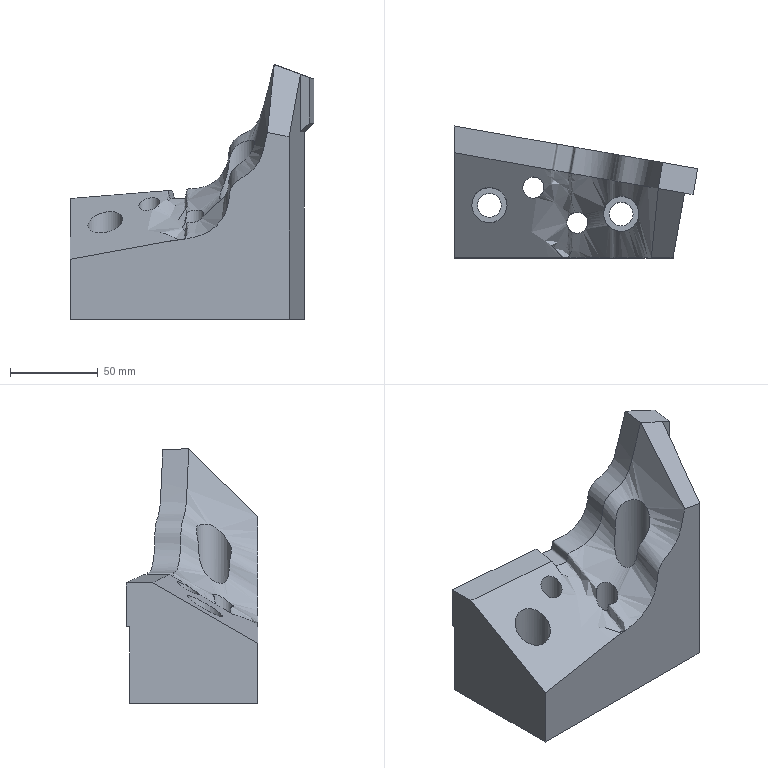Part | NX | features solid 2 | 1 solid | 22 faces | box 138.529 x 75.029 x 144.96 mm | volume 544353 mm3 | plane 12 | cylinder 6 | spline 4 | commonest cylinder face diameters 12 x2 13.5 x2 20 x2